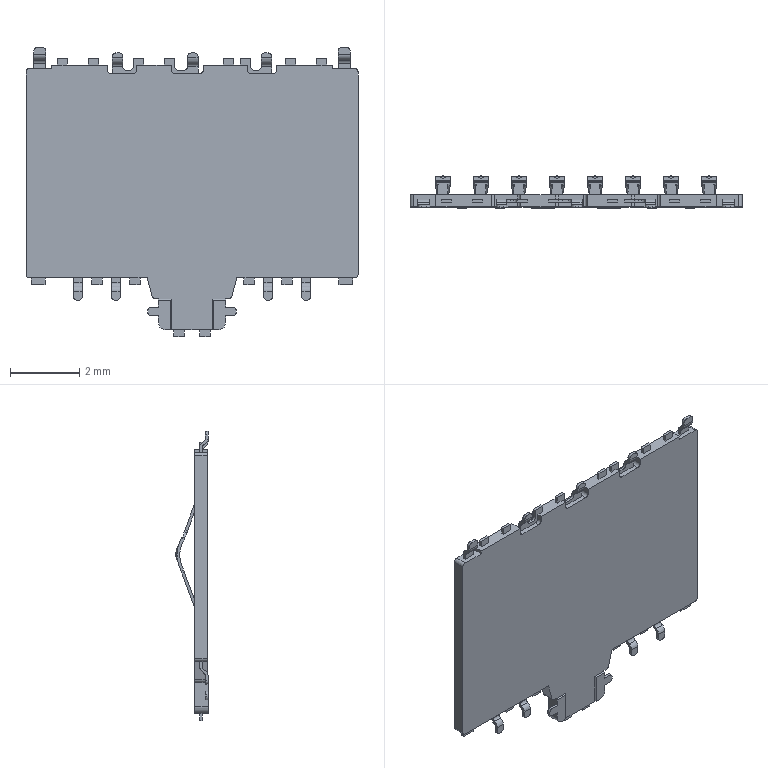Part | Creo | 1 solid | 540 faces | box 9.6 x 0.9296 x 8.36 mm | volume 22.502 mm3 | plane 299 | cylinder 185 | spline 32 | torus 16 | other 8 | commonest cylinder face diameters 0.2 x93 0.36 x18 1.6 x16 1.76 x16 2 x16 1.24 x8